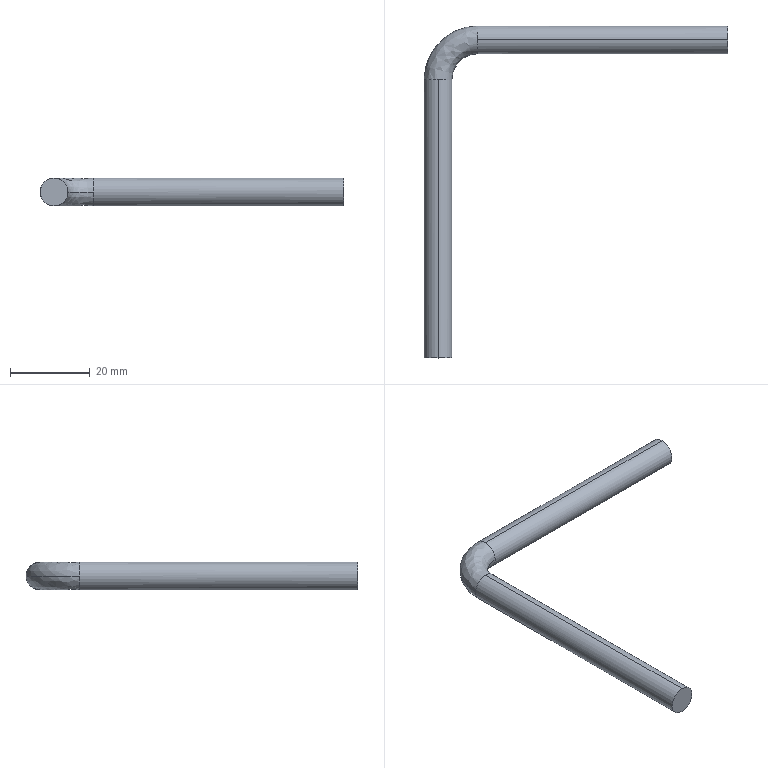Part | SolidWorks | features BaseBody 1 | 1 solid | 8 faces | box 76.4 x 83.5 x 7 mm | volume 5719 mm3 | cylinder 4 | spline 2 | plane 2 | commonest cylinder face diameters 7 x4
STEP:
#1=CARTESIAN_POINT('',(0.,0.,3.328));
#2=VERTEX_POINT('',#1);
#3=CARTESIAN_POINT('',(0.,0.,-3.672));
#4=VERTEX_POINT('',#3);
#5=CARTESIAN_POINT('',(0.,0.,-0.1715));
#6=DIRECTION('',(0.,1.,0.));
#7=DIRECTION('',(0.,0.,1.));
#8=AXIS2_PLACEMENT_3D('',#5,#6,#7);
#9=CIRCLE('',#8,3.5);
#10=EDGE_CURVE('',#2,#4,#9,.T.);
#11=ORIENTED_EDGE('',*,*,#10,.T.);
#12=CARTESIAN_POINT('',(0.,70.,-3.672));
#13=VERTEX_POINT('',#12);
#14=CARTESIAN_POINT('',(0.,0.,-3.672));
#15=DIRECTION('',(0.,1.,0.));
#16=VECTOR('',#15,1000.);
#17=LINE('',#14,#16);
#18=EDGE_CURVE('',#4,#13,#17,.T.);
#19=ORIENTED_EDGE('',*,*,#18,.T.);
#20=CARTESIAN_POINT('',(3.5,70.,-0.1715));
#21=VERTEX_POINT('',#20);
#22=CARTESIAN_POINT('',(0.,70.,-0.1715));
#23=DIRECTION('',(0.,-1.,0.));
#24=DIRECTION('',(0.,0.,1.));
#25=AXIS2_PLACEMENT_3D('',#22,#23,#24);
#26=CIRCLE('',#25,3.5);
#27=EDGE_CURVE('',#13,#21,#26,.T.);
#28=ORIENTED_EDGE('',*,*,#27,.T.);
#29=CARTESIAN_POINT('',(0.,70.,3.328));
#30=VERTEX_POINT('',#29);
#31=CARTESIAN_POINT('',(0.,70.,-0.1715));
#32=DIRECTION('',(0.,-1.,0.));
#33=DIRECTION('',(0.,0.,1.));
#34=AXIS2_PLACEMENT_3D('',#31,#32,#33);
#35=CIRCLE('',#34,3.5);
#36=EDGE_CURVE('',#21,#30,#35,.T.);
#37=ORIENTED_EDGE('',*,*,#36,.T.);
#38=CARTESIAN_POINT('',(0.,0.,3.328));
#39=DIRECTION('',(0.,1.,0.));
#40=VECTOR('',#39,1000.);
#41=LINE('',#38,#40);
#42=EDGE_CURVE('',#2,#30,#41,.T.);
#43=ORIENTED_EDGE('',*,*,#42,.F.);
#44=EDGE_LOOP('',(#11,#19,#28,#37,#43));
#45=FACE_OUTER_BOUND('',#44,.T.);
#46=CARTESIAN_POINT('',(0.,0.,-0.1715));
#47=DIRECTION('',(0.,1.,0.));
#48=DIRECTION('',(0.,0.,1.));
#49=AXIS2_PLACEMENT_3D('',#46,#47,#48);
#50=CYLINDRICAL_SURFACE('',#49,3.5);
#51=ADVANCED_FACE('',(#45),#50,.T.);
#52=ORIENTED_EDGE('',*,*,#36,.F.);
#53=CARTESIAN_POINT('',(10.,76.5,-0.1715));
#54=VERTEX_POINT('',#53);
#55=CARTESIAN_POINT('',(10.,70.,-0.1715));
#56=DIRECTION('',(0.,0.,-1.));
#57=DIRECTION('',(-1.,0.,0.));
#58=AXIS2_PLACEMENT_3D('',#55,#56,#57);
#59=CIRCLE('',#58,6.5);
#60=EDGE_CURVE('',#21,#54,#59,.T.);
#61=ORIENTED_EDGE('',*,*,#60,.T.);
#62=CARTESIAN_POINT('',(10.,80.,3.328));
#63=VERTEX_POINT('',#62);
#64=CARTESIAN_POINT('',(10.,80.,-0.1715));
#65=DIRECTION('',(-1.,0.,0.));
#66=DIRECTION('',(0.,1.,0.));
#67=AXIS2_PLACEMENT_3D('',#64,#65,#66);
#68=CIRCLE('',#67,3.5);
#69=EDGE_CURVE('',#54,#63,#68,.T.);
#70=ORIENTED_EDGE('',*,*,#69,.T.);
#71=CARTESIAN_POINT('',(10.,83.5,-0.1715));
#72=VERTEX_POINT('',#71);
#73=CARTESIAN_POINT('',(10.,80.,-0.1715));
#74=DIRECTION('',(-1.,0.,0.));
#75=DIRECTION('',(0.,1.,0.));
#76=AXIS2_PLACEMENT_3D('',#73,#74,#75);
#77=CIRCLE('',#76,3.5);
#78=EDGE_CURVE('',#63,#72,#77,.T.);
#79=ORIENTED_EDGE('',*,*,#78,.T.);
#80=CARTESIAN_POINT('',(-3.5,70.,-0.1715));
#81=VERTEX_POINT('',#80);
#82=CARTESIAN_POINT('',(10.,70.,-0.1715));
#83=DIRECTION('',(0.,0.,-1.));
#84=DIRECTION('',(-1.,0.,0.));
#85=AXIS2_PLACEMENT_3D('',#82,#83,#84);
#86=CIRCLE('',#85,13.5);
#87=EDGE_CURVE('',#81,#72,#86,.T.);
#88=ORIENTED_EDGE('',*,*,#87,.F.);
#89=CARTESIAN_POINT('',(0.,70.,-0.1715));
#90=DIRECTION('',(0.,-1.,0.));
#91=DIRECTION('',(0.,0.,1.));
#92=AXIS2_PLACEMENT_3D('',#89,#90,#91);
#93=CIRCLE('',#92,3.5);
#94=EDGE_CURVE('',#30,#81,#93,.T.);
#95=ORIENTED_EDGE('',*,*,#94,.F.);
#96=EDGE_LOOP('',(#52,#61,#70,#79,#88,#95));
#97=FACE_OUTER_BOUND('',#96,.T.);
#98=CARTESIAN_POINT('',(-3.5,70.,-0.1715));
#99=CARTESIAN_POINT('',(-3.5,77.908,-0.1715));
#100=CARTESIAN_POINT('',(2.092,83.5,-0.1715));
#101=CARTESIAN_POINT('',(10.,83.5,-0.1715));
#102=CARTESIAN_POINT('',(-3.5,70.,6.828));
#103=CARTESIAN_POINT('',(-3.5,77.908,6.828));
#104=CARTESIAN_POINT('',(2.092,83.5,6.828));
#105=CARTESIAN_POINT('',(10.,83.5,6.828));
#106=CARTESIAN_POINT('',(3.5,70.,6.828));
#107=CARTESIAN_POINT('',(3.5,73.808,6.828));
#108=CARTESIAN_POINT('',(6.192,76.5,6.828));
#109=CARTESIAN_POINT('',(10.,76.5,6.828));
#110=CARTESIAN_POINT('',(3.5,70.,-0.1715));
#111=CARTESIAN_POINT('',(3.5,73.808,-0.1715));
#112=CARTESIAN_POINT('',(6.192,76.5,-0.1715));
#113=CARTESIAN_POINT('',(10.,76.5,-0.1715));
#114=(BOUNDED_SURFACE()B_SPLINE_SURFACE(3,3,((#98,#99,#100,#101),(#102,#103,#104,#105),(#106,#107,#108,#109),(#110,#111,#112,#113)),.UNSPECIFIED.,.F.,.F.,.F.)B_SPLINE_SURFACE_WITH_KNOTS((4,4),(4,4),(0.,1.),(0.,1.),.UNSPECIFIED.)GEOMETRIC_REPRESENTATION_ITEM()RATIONAL_B_SPLINE_SURFACE(((1.,0.8047,0.8047,1.),(0.3333,0.2682,0.2682,0.3333),(0.3333,0.2682,0.2682,0.3333),(1.,0.8047,0.8047,1.)))REPRESENTATION_ITEM('')SURFACE());
#115=ADVANCED_FACE('',(#97),#114,.T.);
#116=ORIENTED_EDGE('',*,*,#78,.F.);
#117=CARTESIAN_POINT('',(72.9,80.,3.328));
#118=VERTEX_POINT('',#117);
#119=CARTESIAN_POINT('',(10.,80.,3.328));
#120=DIRECTION('',(1.,0.,0.));
#121=VECTOR('',#120,1000.);
#122=LINE('',#119,#121);
#123=EDGE_CURVE('',#63,#118,#122,.T.);
#124=ORIENTED_EDGE('',*,*,#123,.T.);
#125=CARTESIAN_POINT('',(72.9,80.,-3.672));
#126=VERTEX_POINT('',#125);
#127=CARTESIAN_POINT('',(72.9,80.,-0.1715));
#128=DIRECTION('',(-1.,0.,0.));
#129=DIRECTION('',(0.,0.,-1.));
#130=AXIS2_PLACEMENT_3D('',#127,#128,#129);
#131=CIRCLE('',#130,3.5);
#132=EDGE_CURVE('',#118,#126,#131,.T.);
#133=ORIENTED_EDGE('',*,*,#132,.T.);
#134=CARTESIAN_POINT('',(10.,80.,-3.672));
#135=VERTEX_POINT('',#134);
#136=CARTESIAN_POINT('',(10.,80.,-3.672));
#137=DIRECTION('',(1.,0.,0.));
#138=VECTOR('',#137,1000.);
#139=LINE('',#136,#138);
#140=EDGE_CURVE('',#135,#126,#139,.T.);
#141=ORIENTED_EDGE('',*,*,#140,.F.);
#142=CARTESIAN_POINT('',(10.,80.,-0.1715));
#143=DIRECTION('',(-1.,0.,0.));
#144=DIRECTION('',(0.,1.,0.));
#145=AXIS2_PLACEMENT_3D('',#142,#143,#144);
#146=CIRCLE('',#145,3.5);
#147=EDGE_CURVE('',#72,#135,#146,.T.);
#148=ORIENTED_EDGE('',*,*,#147,.F.);
#149=EDGE_LOOP('',(#116,#124,#133,#141,#148));
#150=FACE_OUTER_BOUND('',#149,.T.);
#151=CARTESIAN_POINT('',(10.,80.,-0.1715));
#152=DIRECTION('',(1.,0.,0.));
#153=DIRECTION('',(0.,0.,-1.));
#154=AXIS2_PLACEMENT_3D('',#151,#152,#153);
#155=CYLINDRICAL_SURFACE('',#154,3.5);
#156=ADVANCED_FACE('',(#150),#155,.T.);
#157=ORIENTED_EDGE('',*,*,#18,.F.);
#158=CARTESIAN_POINT('',(0.,0.,-0.1715));
#159=DIRECTION('',(0.,1.,0.));
#160=DIRECTION('',(0.,0.,1.));
#161=AXIS2_PLACEMENT_3D('',#158,#159,#160);
#162=CIRCLE('',#161,3.5);
#163=EDGE_CURVE('',#4,#2,#162,.T.);
#164=ORIENTED_EDGE('',*,*,#163,.T.);
#165=ORIENTED_EDGE('',*,*,#42,.T.);
#166=ORIENTED_EDGE('',*,*,#94,.T.);
#167=CARTESIAN_POINT('',(0.,70.,-0.1715));
#168=DIRECTION('',(0.,-1.,0.));
#169=DIRECTION('',(0.,0.,1.));
#170=AXIS2_PLACEMENT_3D('',#167,#168,#169);
#171=CIRCLE('',#170,3.5);
#172=EDGE_CURVE('',#81,#13,#171,.T.);
#173=ORIENTED_EDGE('',*,*,#172,.T.);
#174=EDGE_LOOP('',(#157,#164,#165,#166,#173));
#175=FACE_OUTER_BOUND('',#174,.T.);
#176=CARTESIAN_POINT('',(0.,0.,-0.1715));
#177=DIRECTION('',(0.,1.,0.));
#178=DIRECTION('',(0.,0.,1.));
#179=AXIS2_PLACEMENT_3D('',#176,#177,#178);
#180=CYLINDRICAL_SURFACE('',#179,3.5);
#181=ADVANCED_FACE('',(#175),#180,.T.);
#182=ORIENTED_EDGE('',*,*,#60,.F.);
#183=ORIENTED_EDGE('',*,*,#27,.F.);
#184=ORIENTED_EDGE('',*,*,#172,.F.);
#185=ORIENTED_EDGE('',*,*,#87,.T.);
#186=ORIENTED_EDGE('',*,*,#147,.T.);
#187=CARTESIAN_POINT('',(10.,80.,-0.1715));
#188=DIRECTION('',(-1.,0.,0.));
#189=DIRECTION('',(0.,1.,0.));
#190=AXIS2_PLACEMENT_3D('',#187,#188,#189);
#191=CIRCLE('',#190,3.5);
#192=EDGE_CURVE('',#135,#54,#191,.T.);
#193=ORIENTED_EDGE('',*,*,#192,.T.);
#194=EDGE_LOOP('',(#182,#183,#184,#185,#186,#193));
#195=FACE_OUTER_BOUND('',#194,.T.);
#196=CARTESIAN_POINT('',(3.5,70.,-0.1715));
#197=CARTESIAN_POINT('',(3.5,73.808,-0.1715));
#198=CARTESIAN_POINT('',(6.192,76.5,-0.1715));
#199=CARTESIAN_POINT('',(10.,76.5,-0.1715));
#200=CARTESIAN_POINT('',(3.5,70.,-7.172));
#201=CARTESIAN_POINT('',(3.5,73.808,-7.172));
#202=CARTESIAN_POINT('',(6.192,76.5,-7.172));
#203=CARTESIAN_POINT('',(10.,76.5,-7.172));
#204=CARTESIAN_POINT('',(-3.5,70.,-7.172));
#205=CARTESIAN_POINT('',(-3.5,77.908,-7.172));
#206=CARTESIAN_POINT('',(2.092,83.5,-7.172));
#207=CARTESIAN_POINT('',(10.,83.5,-7.172));
#208=CARTESIAN_POINT('',(-3.5,70.,-0.1715));
#209=CARTESIAN_POINT('',(-3.5,77.908,-0.1715));
#210=CARTESIAN_POINT('',(2.092,83.5,-0.1715));
#211=CARTESIAN_POINT('',(10.,83.5,-0.1715));
#212=(BOUNDED_SURFACE()B_SPLINE_SURFACE(3,3,((#196,#197,#198,#199),(#200,#201,#202,#203),(#204,#205,#206,#207),(#208,#209,#210,#211)),.UNSPECIFIED.,.F.,.F.,.F.)B_SPLINE_SURFACE_WITH_KNOTS((4,4),(4,4),(0.,1.),(0.,1.),.UNSPECIFIED.)GEOMETRIC_REPRESENTATION_ITEM()RATIONAL_B_SPLINE_SURFACE(((1.,0.8047,0.8047,1.),(0.3333,0.2682,0.2682,0.3333),(0.3333,0.2682,0.2682,0.3333),(1.,0.8047,0.8047,1.)))REPRESENTATION_ITEM('')SURFACE());
#213=ADVANCED_FACE('',(#195),#212,.T.);
#214=ORIENTED_EDGE('',*,*,#10,.F.);
#215=ORIENTED_EDGE('',*,*,#163,.F.);
#216=EDGE_LOOP('',(#214,#215));
#217=FACE_OUTER_BOUND('',#216,.T.);
#218=CARTESIAN_POINT('',(0.,0.,-0.1715));
#219=DIRECTION('',(0.,1.,0.));
#220=DIRECTION('',(0.,0.,1.));
#221=AXIS2_PLACEMENT_3D('',#218,#219,#220);
#222=PLANE('',#221);
#223=ADVANCED_FACE('',(#217),#222,.F.);
#224=ORIENTED_EDGE('',*,*,#123,.F.);
#225=ORIENTED_EDGE('',*,*,#69,.F.);
#226=ORIENTED_EDGE('',*,*,#192,.F.);
#227=ORIENTED_EDGE('',*,*,#140,.T.);
#228=CARTESIAN_POINT('',(72.9,80.,-0.1715));
#229=DIRECTION('',(-1.,0.,0.));
#230=DIRECTION('',(0.,0.,-1.));
#231=AXIS2_PLACEMENT_3D('',#228,#229,#230);
#232=CIRCLE('',#231,3.5);
#233=EDGE_CURVE('',#126,#118,#232,.T.);
#234=ORIENTED_EDGE('',*,*,#233,.T.);
#235=EDGE_LOOP('',(#224,#225,#226,#227,#234));
#236=FACE_OUTER_BOUND('',#235,.T.);
#237=CARTESIAN_POINT('',(10.,80.,-0.1715));
#238=DIRECTION('',(1.,0.,0.));
#239=DIRECTION('',(0.,0.,-1.));
#240=AXIS2_PLACEMENT_3D('',#237,#238,#239);
#241=CYLINDRICAL_SURFACE('',#240,3.5);
#242=ADVANCED_FACE('',(#236),#241,.T.);
#243=ORIENTED_EDGE('',*,*,#233,.F.);
#244=ORIENTED_EDGE('',*,*,#132,.F.);
#245=EDGE_LOOP('',(#243,#244));
#246=FACE_OUTER_BOUND('',#245,.T.);
#247=CARTESIAN_POINT('',(72.9,80.,-0.1715));
#248=DIRECTION('',(1.,0.,0.));
#249=DIRECTION('',(0.,0.,-1.));
#250=AXIS2_PLACEMENT_3D('',#247,#248,#249);
#251=PLANE('',#250);
#252=ADVANCED_FACE('',(#246),#251,.T.);
#253=CLOSED_SHELL('',(#51,#115,#156,#181,#213,#223,#242,#252));
#254=MANIFOLD_SOLID_BREP('',#253);
#255=CARTESIAN_POINT('',(0.,0.,0.));
#256=DIRECTION('',(0.,0.,1.));
#257=DIRECTION('',(1.,0.,0.));
#258=AXIS2_PLACEMENT_3D('',#255,#256,#257);
#259=(LENGTH_UNIT()NAMED_UNIT(*)SI_UNIT(.MILLI.,.METRE.));
#260=UNCERTAINTY_MEASURE_WITH_UNIT(LENGTH_MEASURE(0.00001),#259,'','');
#261=(NAMED_UNIT(*)PLANE_ANGLE_UNIT()SI_UNIT($,.RADIAN.));
#262=(NAMED_UNIT(*)SI_UNIT($,.STERADIAN.)SOLID_ANGLE_UNIT());
#263=(GEOMETRIC_REPRESENTATION_CONTEXT(3)GLOBAL_UNCERTAINTY_ASSIGNED_CONTEXT((#260))GLOBAL_UNIT_ASSIGNED_CONTEXT((#259,#261,#262))REPRESENTATION_CONTEXT('',''));
#264=ADVANCED_BREP_SHAPE_REPRESENTATION('',(#254,#258),#263);